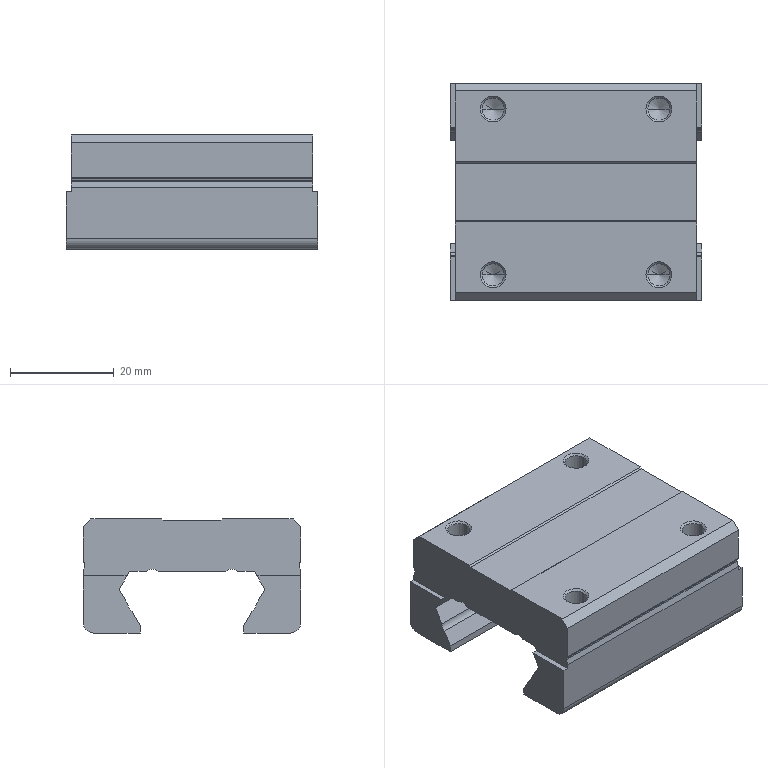Part | NX | 1 solid | 92 faces | box 48.6 x 42 x 22 mm | volume 28885 mm3 | plane 44 | cylinder 32 | cone 16 | commonest cylinder face diameters 4.29 x8 4.3 x8 5 x8 3.3 x4 1 x2 4 x2